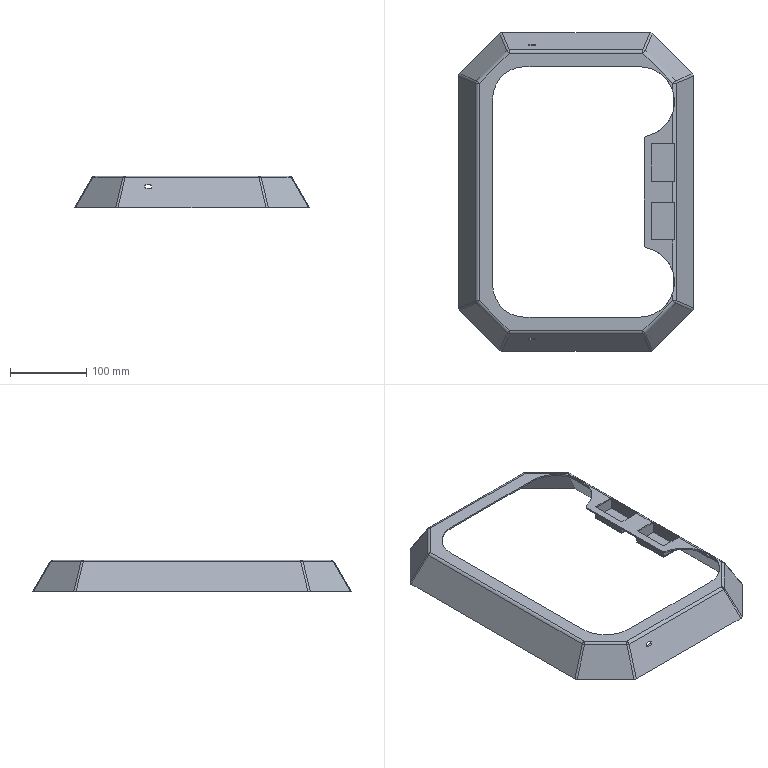Part | NX | features 模具.stp<1>[1] 2 | 1 solid | 113 faces | box 308.497 x 418.497 x 42 mm | volume 188000 mm3 | plane 71 | cylinder 26 | spline 8 | sphere 8 | commonest cylinder face diameters 10 x18 96.927 x4 85 x2 91.927 x2